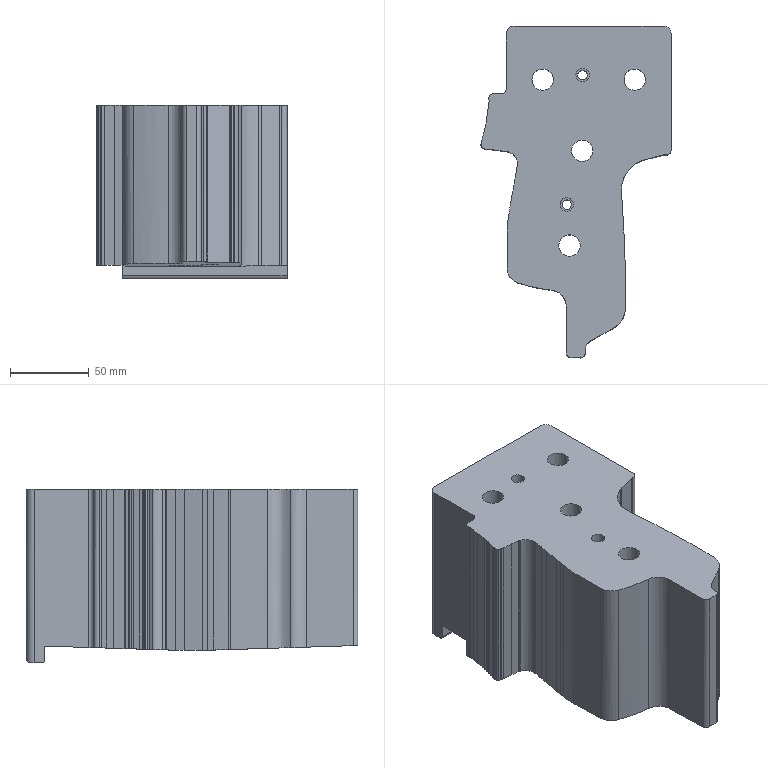Part | STEP file | lll_id3202_x_t | 1 solid | 110 faces | box 120.313 x 210 x 110 mm | volume 1542446 mm3 | cylinder 86 | plane 22 | cone 2 | commonest cylinder face diameters 6 x10 13.509 x4 20.007 x4 20 x3 8.5 x2 10 x2